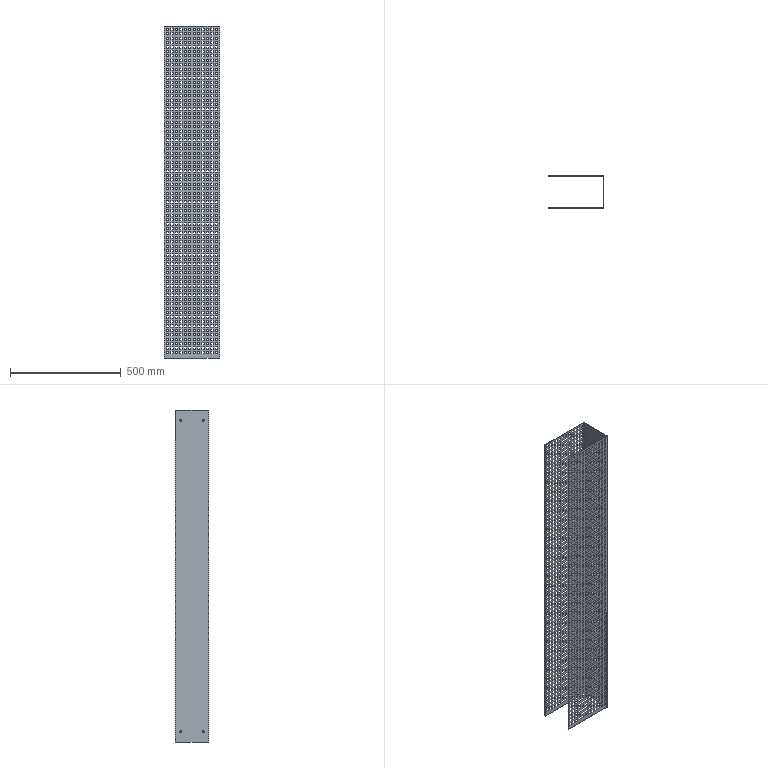Part | SolidWorks | features EdgeFlange 1, FlatPattern 1, HoleWzd 1, ICE 1, LPattern 1, SMBaseFlange 1, SheetMetal 1 | 1 solid | 7134 faces | volume 1186097 mm3 | plane 7122 | cylinder 12 | commonest cylinder face diameters 9 x8 1.473 x2 4.473 x2